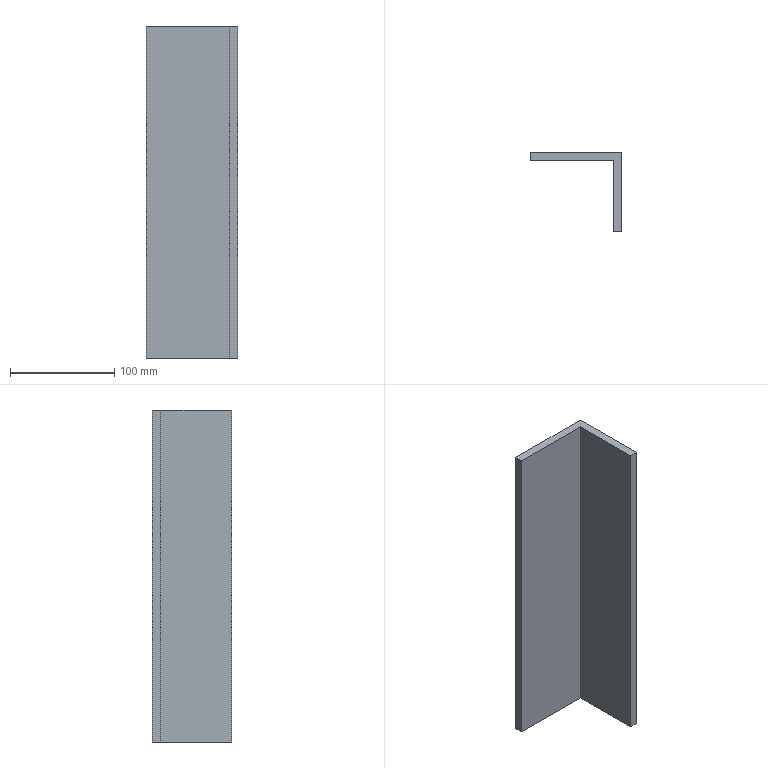Part | SolidWorks | features ICE 3, Extrusion 1 | 1 solid | 8 faces | box 88 x 76 x 318 mm | volume 396864 mm3 | plane 8
STEP:
#1=CARTESIAN_POINT('',(8.,-8.,310.));
#2=VERTEX_POINT('',#1);
#3=CARTESIAN_POINT('',(8.,68.,310.));
#4=VERTEX_POINT('',#3);
#5=CARTESIAN_POINT('',(8.,0.,310.));
#6=DIRECTION('',(0.,1.,0.));
#7=VECTOR('',#6,1000.);
#8=LINE('',#5,#7);
#9=EDGE_CURVE('',#2,#4,#8,.T.);
#10=ORIENTED_EDGE('',*,*,#9,.F.);
#11=CARTESIAN_POINT('',(8.,-8.,-8.));
#12=VERTEX_POINT('',#11);
#13=CARTESIAN_POINT('',(8.,-8.,-8.));
#14=DIRECTION('',(0.,0.,1.));
#15=VECTOR('',#14,1000.);
#16=LINE('',#13,#15);
#17=EDGE_CURVE('',#12,#2,#16,.T.);
#18=ORIENTED_EDGE('',*,*,#17,.F.);
#19=CARTESIAN_POINT('',(8.,68.,-8.));
#20=VERTEX_POINT('',#19);
#21=CARTESIAN_POINT('',(8.,68.,-8.));
#22=DIRECTION('',(0.,-1.,0.));
#23=VECTOR('',#22,1000.);
#24=LINE('',#21,#23);
#25=EDGE_CURVE('',#20,#12,#24,.T.);
#26=ORIENTED_EDGE('',*,*,#25,.F.);
#27=CARTESIAN_POINT('',(8.,68.,300.));
#28=DIRECTION('',(0.,0.,-1.));
#29=VECTOR('',#28,1000.);
#30=LINE('',#27,#29);
#31=EDGE_CURVE('',#4,#20,#30,.T.);
#32=ORIENTED_EDGE('',*,*,#31,.F.);
#33=EDGE_LOOP('',(#10,#18,#26,#32));
#34=FACE_OUTER_BOUND('',#33,.T.);
#35=CARTESIAN_POINT('',(8.,0.,300.));
#36=DIRECTION('',(-1.,0.,0.));
#37=DIRECTION('',(0.,0.,1.));
#38=AXIS2_PLACEMENT_3D('',#35,#36,#37);
#39=PLANE('',#38);
#40=ADVANCED_FACE('',(#34),#39,.F.);
#41=ORIENTED_EDGE('',*,*,#31,.T.);
#42=CARTESIAN_POINT('',(-80.,68.,-8.));
#43=VERTEX_POINT('',#42);
#44=CARTESIAN_POINT('',(-80.,68.,-8.));
#45=DIRECTION('',(1.,0.,0.));
#46=VECTOR('',#45,1000.);
#47=LINE('',#44,#46);
#48=EDGE_CURVE('',#43,#20,#47,.T.);
#49=ORIENTED_EDGE('',*,*,#48,.F.);
#50=CARTESIAN_POINT('',(-80.,68.,310.));
#51=VERTEX_POINT('',#50);
#52=CARTESIAN_POINT('',(-80.,68.,300.));
#53=DIRECTION('',(0.,0.,-1.));
#54=VECTOR('',#53,1000.);
#55=LINE('',#52,#54);
#56=EDGE_CURVE('',#51,#43,#55,.T.);
#57=ORIENTED_EDGE('',*,*,#56,.F.);
#58=CARTESIAN_POINT('',(8.,68.,310.));
#59=DIRECTION('',(-1.,0.,0.));
#60=VECTOR('',#59,1000.);
#61=LINE('',#58,#60);
#62=EDGE_CURVE('',#4,#51,#61,.T.);
#63=ORIENTED_EDGE('',*,*,#62,.F.);
#64=EDGE_LOOP('',(#41,#49,#57,#63));
#65=FACE_OUTER_BOUND('',#64,.T.);
#66=CARTESIAN_POINT('',(8.,68.,300.));
#67=DIRECTION('',(0.,-1.,0.));
#68=DIRECTION('',(0.,0.,-1.));
#69=AXIS2_PLACEMENT_3D('',#66,#67,#68);
#70=PLANE('',#69);
#71=ADVANCED_FACE('',(#65),#70,.F.);
#72=ORIENTED_EDGE('',*,*,#56,.T.);
#73=CARTESIAN_POINT('',(-80.,60.,-8.));
#74=VERTEX_POINT('',#73);
#75=CARTESIAN_POINT('',(-80.,60.,-8.));
#76=DIRECTION('',(0.,1.,0.));
#77=VECTOR('',#76,1000.);
#78=LINE('',#75,#77);
#79=EDGE_CURVE('',#74,#43,#78,.T.);
#80=ORIENTED_EDGE('',*,*,#79,.F.);
#81=CARTESIAN_POINT('',(-80.,60.,310.));
#82=VERTEX_POINT('',#81);
#83=CARTESIAN_POINT('',(-80.,60.,300.));
#84=DIRECTION('',(0.,0.,-1.));
#85=VECTOR('',#84,1000.);
#86=LINE('',#83,#85);
#87=EDGE_CURVE('',#82,#74,#86,.T.);
#88=ORIENTED_EDGE('',*,*,#87,.F.);
#89=CARTESIAN_POINT('',(-80.,68.,310.));
#90=DIRECTION('',(0.,-1.,0.));
#91=VECTOR('',#90,1000.);
#92=LINE('',#89,#91);
#93=EDGE_CURVE('',#51,#82,#92,.T.);
#94=ORIENTED_EDGE('',*,*,#93,.F.);
#95=EDGE_LOOP('',(#72,#80,#88,#94));
#96=FACE_OUTER_BOUND('',#95,.T.);
#97=CARTESIAN_POINT('',(-80.,60.,300.));
#98=DIRECTION('',(1.,0.,0.));
#99=DIRECTION('',(0.,0.,-1.));
#100=AXIS2_PLACEMENT_3D('',#97,#98,#99);
#101=PLANE('',#100);
#102=ADVANCED_FACE('',(#96),#101,.F.);
#103=ORIENTED_EDGE('',*,*,#87,.T.);
#104=CARTESIAN_POINT('',(0.,60.,-8.));
#105=VERTEX_POINT('',#104);
#106=CARTESIAN_POINT('',(0.,60.,-8.));
#107=DIRECTION('',(-1.,0.,0.));
#108=VECTOR('',#107,1000.);
#109=LINE('',#106,#108);
#110=EDGE_CURVE('',#105,#74,#109,.T.);
#111=ORIENTED_EDGE('',*,*,#110,.F.);
#112=CARTESIAN_POINT('',(0.,60.,310.));
#113=VERTEX_POINT('',#112);
#114=CARTESIAN_POINT('',(0.,60.,300.));
#115=DIRECTION('',(0.,0.,-1.));
#116=VECTOR('',#115,1000.);
#117=LINE('',#114,#116);
#118=EDGE_CURVE('',#113,#105,#117,.T.);
#119=ORIENTED_EDGE('',*,*,#118,.F.);
#120=CARTESIAN_POINT('',(-80.,60.,310.));
#121=DIRECTION('',(1.,0.,0.));
#122=VECTOR('',#121,1000.);
#123=LINE('',#120,#122);
#124=EDGE_CURVE('',#82,#113,#123,.T.);
#125=ORIENTED_EDGE('',*,*,#124,.F.);
#126=EDGE_LOOP('',(#103,#111,#119,#125));
#127=FACE_OUTER_BOUND('',#126,.T.);
#128=CARTESIAN_POINT('',(0.,60.,300.));
#129=DIRECTION('',(0.,1.,0.));
#130=DIRECTION('',(-1.,0.,0.));
#131=AXIS2_PLACEMENT_3D('',#128,#129,#130);
#132=PLANE('',#131);
#133=ADVANCED_FACE('',(#127),#132,.F.);
#134=ORIENTED_EDGE('',*,*,#118,.T.);
#135=CARTESIAN_POINT('',(0.,-8.,-8.));
#136=VERTEX_POINT('',#135);
#137=CARTESIAN_POINT('',(0.,0.,-8.));
#138=DIRECTION('',(0.,1.,0.));
#139=VECTOR('',#138,1000.);
#140=LINE('',#137,#139);
#141=EDGE_CURVE('',#136,#105,#140,.T.);
#142=ORIENTED_EDGE('',*,*,#141,.F.);
#143=CARTESIAN_POINT('',(0.,-8.,310.));
#144=VERTEX_POINT('',#143);
#145=CARTESIAN_POINT('',(0.,-8.,310.));
#146=DIRECTION('',(0.,0.,-1.));
#147=VECTOR('',#146,1000.);
#148=LINE('',#145,#147);
#149=EDGE_CURVE('',#144,#136,#148,.T.);
#150=ORIENTED_EDGE('',*,*,#149,.F.);
#151=CARTESIAN_POINT('',(0.,60.,310.));
#152=DIRECTION('',(0.,-1.,0.));
#153=VECTOR('',#152,1000.);
#154=LINE('',#151,#153);
#155=EDGE_CURVE('',#113,#144,#154,.T.);
#156=ORIENTED_EDGE('',*,*,#155,.F.);
#157=EDGE_LOOP('',(#134,#142,#150,#156));
#158=FACE_OUTER_BOUND('',#157,.T.);
#159=CARTESIAN_POINT('',(0.,0.,300.));
#160=DIRECTION('',(1.,0.,0.));
#161=DIRECTION('',(0.,0.,-1.));
#162=AXIS2_PLACEMENT_3D('',#159,#160,#161);
#163=PLANE('',#162);
#164=ADVANCED_FACE('',(#158),#163,.F.);
#165=ORIENTED_EDGE('',*,*,#155,.T.);
#166=CARTESIAN_POINT('',(8.,-8.,310.));
#167=DIRECTION('',(-1.,0.,0.));
#168=VECTOR('',#167,1000.);
#169=LINE('',#166,#168);
#170=EDGE_CURVE('',#2,#144,#169,.T.);
#171=ORIENTED_EDGE('',*,*,#170,.F.);
#172=ORIENTED_EDGE('',*,*,#9,.T.);
#173=ORIENTED_EDGE('',*,*,#62,.T.);
#174=ORIENTED_EDGE('',*,*,#93,.T.);
#175=ORIENTED_EDGE('',*,*,#124,.T.);
#176=EDGE_LOOP('',(#165,#171,#172,#173,#174,#175));
#177=FACE_OUTER_BOUND('',#176,.T.);
#178=CARTESIAN_POINT('',(0.,0.,310.));
#179=DIRECTION('',(0.,0.,1.));
#180=DIRECTION('',(1.,0.,0.));
#181=AXIS2_PLACEMENT_3D('',#178,#179,#180);
#182=PLANE('',#181);
#183=ADVANCED_FACE('',(#177),#182,.T.);
#184=ORIENTED_EDGE('',*,*,#25,.T.);
#185=CARTESIAN_POINT('',(0.,-8.,-8.));
#186=DIRECTION('',(1.,0.,0.));
#187=VECTOR('',#186,1000.);
#188=LINE('',#185,#187);
#189=EDGE_CURVE('',#136,#12,#188,.T.);
#190=ORIENTED_EDGE('',*,*,#189,.F.);
#191=ORIENTED_EDGE('',*,*,#141,.T.);
#192=ORIENTED_EDGE('',*,*,#110,.T.);
#193=ORIENTED_EDGE('',*,*,#79,.T.);
#194=ORIENTED_EDGE('',*,*,#48,.T.);
#195=EDGE_LOOP('',(#184,#190,#191,#192,#193,#194));
#196=FACE_OUTER_BOUND('',#195,.T.);
#197=CARTESIAN_POINT('',(0.,0.,-8.));
#198=DIRECTION('',(0.,0.,-1.));
#199=DIRECTION('',(-1.,0.,0.));
#200=AXIS2_PLACEMENT_3D('',#197,#198,#199);
#201=PLANE('',#200);
#202=ADVANCED_FACE('',(#196),#201,.T.);
#203=ORIENTED_EDGE('',*,*,#170,.T.);
#204=ORIENTED_EDGE('',*,*,#149,.T.);
#205=ORIENTED_EDGE('',*,*,#189,.T.);
#206=ORIENTED_EDGE('',*,*,#17,.T.);
#207=EDGE_LOOP('',(#203,#204,#205,#206));
#208=FACE_OUTER_BOUND('',#207,.T.);
#209=CARTESIAN_POINT('',(0.,-8.,0.));
#210=DIRECTION('',(0.,-1.,0.));
#211=DIRECTION('',(0.,0.,-1.));
#212=AXIS2_PLACEMENT_3D('',#209,#210,#211);
#213=PLANE('',#212);
#214=ADVANCED_FACE('',(#208),#213,.T.);
#215=CLOSED_SHELL('',(#40,#71,#102,#133,#164,#183,#202,#214));
#216=MANIFOLD_SOLID_BREP('',#215);
#217=CARTESIAN_POINT('',(0.,0.,0.));
#218=DIRECTION('',(0.,0.,1.));
#219=DIRECTION('',(1.,0.,0.));
#220=AXIS2_PLACEMENT_3D('',#217,#218,#219);
#221=(LENGTH_UNIT()NAMED_UNIT(*)SI_UNIT(.MILLI.,.METRE.));
#222=UNCERTAINTY_MEASURE_WITH_UNIT(LENGTH_MEASURE(0.00001),#221,'','');
#223=(NAMED_UNIT(*)PLANE_ANGLE_UNIT()SI_UNIT($,.RADIAN.));
#224=(NAMED_UNIT(*)SI_UNIT($,.STERADIAN.)SOLID_ANGLE_UNIT());
#225=(GEOMETRIC_REPRESENTATION_CONTEXT(3)GLOBAL_UNCERTAINTY_ASSIGNED_CONTEXT((#222))GLOBAL_UNIT_ASSIGNED_CONTEXT((#221,#223,#224))REPRESENTATION_CONTEXT('',''));
#226=ADVANCED_BREP_SHAPE_REPRESENTATION('',(#216,#220),#225);